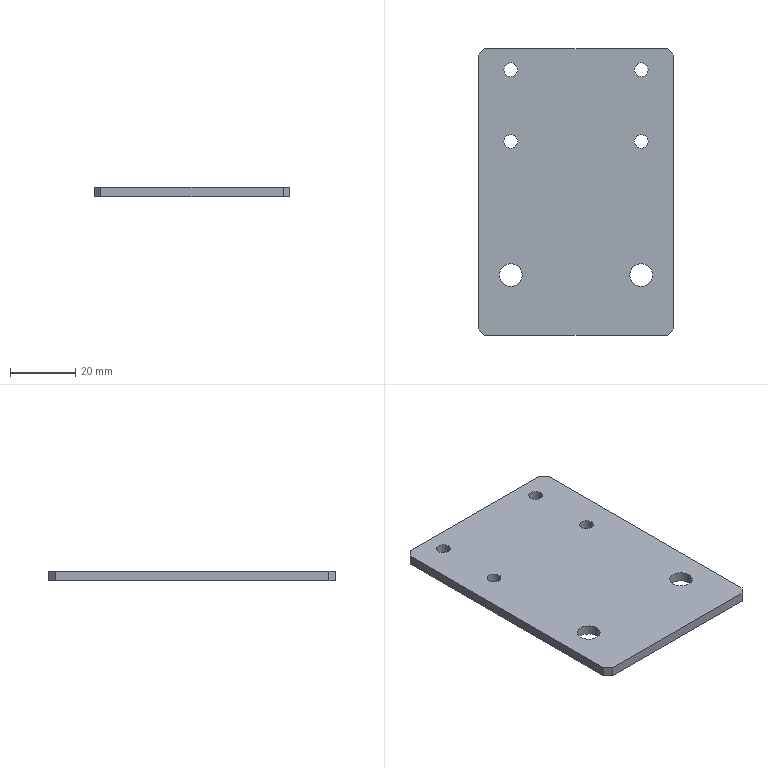Part | NX | features BREP 1 | 1 solid | 22 faces | box 60 x 88 x 3 mm | volume 15419 mm3 | cylinder 12 | plane 10 | commonest cylinder face diameters 4.2 x8 7 x4
STEP:
#1=CARTESIAN_POINT('',(30.,-42.,-3.));
#2=VERTEX_POINT('',#1);
#3=CARTESIAN_POINT('',(28.,-44.,-3.));
#4=VERTEX_POINT('',#3);
#5=CARTESIAN_POINT('',(28.,-44.,-3.));
#6=DIRECTION('',(-0.7071,-0.7071,0.));
#7=VECTOR('',#6,1000.);
#8=LINE('',#5,#7);
#9=EDGE_CURVE('',#2,#4,#8,.T.);
#10=ORIENTED_EDGE('',*,*,#9,.F.);
#11=CARTESIAN_POINT('',(30.,-42.,0.));
#12=VERTEX_POINT('',#11);
#13=CARTESIAN_POINT('',(30.,-42.,-3.));
#14=DIRECTION('',(0.,0.,-1.));
#15=VECTOR('',#14,1000.);
#16=LINE('',#13,#15);
#17=EDGE_CURVE('',#12,#2,#16,.T.);
#18=ORIENTED_EDGE('',*,*,#17,.F.);
#19=CARTESIAN_POINT('',(28.,-44.,0.));
#20=VERTEX_POINT('',#19);
#21=CARTESIAN_POINT('',(36.,-36.,0.));
#22=DIRECTION('',(0.7071,0.7071,0.));
#23=VECTOR('',#22,1000.);
#24=LINE('',#21,#23);
#25=EDGE_CURVE('',#20,#12,#24,.T.);
#26=ORIENTED_EDGE('',*,*,#25,.F.);
#27=CARTESIAN_POINT('',(28.,-44.,-3.));
#28=DIRECTION('',(0.,0.,1.));
#29=VECTOR('',#28,1000.);
#30=LINE('',#27,#29);
#31=EDGE_CURVE('',#4,#20,#30,.T.);
#32=ORIENTED_EDGE('',*,*,#31,.F.);
#33=EDGE_LOOP('',(#10,#18,#26,#32));
#34=FACE_BOUND('',#33,.T.);
#35=CARTESIAN_POINT('',(28.,-44.,-3.));
#36=DIRECTION('',(-0.7071,0.7071,0.));
#37=DIRECTION('',(0.,0.,1.));
#38=AXIS2_PLACEMENT_3D('',#35,#36,#37);
#39=PLANE('',#38);
#40=ADVANCED_FACE('',(#34),#39,.F.);
#41=CARTESIAN_POINT('',(-28.,-44.,-3.));
#42=VERTEX_POINT('',#41);
#43=CARTESIAN_POINT('',(-30.,-42.,-3.));
#44=VERTEX_POINT('',#43);
#45=CARTESIAN_POINT('',(-30.,-42.,-3.));
#46=DIRECTION('',(-0.7071,0.7071,0.));
#47=VECTOR('',#46,1000.);
#48=LINE('',#45,#47);
#49=EDGE_CURVE('',#42,#44,#48,.T.);
#50=ORIENTED_EDGE('',*,*,#49,.F.);
#51=CARTESIAN_POINT('',(-28.,-44.,0.));
#52=VERTEX_POINT('',#51);
#53=CARTESIAN_POINT('',(-28.,-44.,-3.));
#54=DIRECTION('',(0.,0.,-1.));
#55=VECTOR('',#54,1000.);
#56=LINE('',#53,#55);
#57=EDGE_CURVE('',#52,#42,#56,.T.);
#58=ORIENTED_EDGE('',*,*,#57,.F.);
#59=CARTESIAN_POINT('',(-30.,-42.,0.));
#60=VERTEX_POINT('',#59);
#61=CARTESIAN_POINT('',(-36.,-36.,0.));
#62=DIRECTION('',(0.7071,-0.7071,0.));
#63=VECTOR('',#62,1000.);
#64=LINE('',#61,#63);
#65=EDGE_CURVE('',#60,#52,#64,.T.);
#66=ORIENTED_EDGE('',*,*,#65,.F.);
#67=CARTESIAN_POINT('',(-30.,-42.,-3.));
#68=DIRECTION('',(0.,0.,1.));
#69=VECTOR('',#68,1000.);
#70=LINE('',#67,#69);
#71=EDGE_CURVE('',#44,#60,#70,.T.);
#72=ORIENTED_EDGE('',*,*,#71,.F.);
#73=EDGE_LOOP('',(#50,#58,#66,#72));
#74=FACE_BOUND('',#73,.T.);
#75=CARTESIAN_POINT('',(-30.,-42.,-3.));
#76=DIRECTION('',(0.7071,0.7071,0.));
#77=DIRECTION('',(0.,0.,1.));
#78=AXIS2_PLACEMENT_3D('',#75,#76,#77);
#79=PLANE('',#78);
#80=ADVANCED_FACE('',(#74),#79,.F.);
#81=CARTESIAN_POINT('',(28.,44.,-3.));
#82=VERTEX_POINT('',#81);
#83=CARTESIAN_POINT('',(30.,42.,-3.));
#84=VERTEX_POINT('',#83);
#85=CARTESIAN_POINT('',(30.,42.,-3.));
#86=DIRECTION('',(0.7071,-0.7071,0.));
#87=VECTOR('',#86,1000.);
#88=LINE('',#85,#87);
#89=EDGE_CURVE('',#82,#84,#88,.T.);
#90=ORIENTED_EDGE('',*,*,#89,.F.);
#91=CARTESIAN_POINT('',(28.,44.,0.));
#92=VERTEX_POINT('',#91);
#93=CARTESIAN_POINT('',(28.,44.,-3.));
#94=DIRECTION('',(0.,0.,-1.));
#95=VECTOR('',#94,1000.);
#96=LINE('',#93,#95);
#97=EDGE_CURVE('',#92,#82,#96,.T.);
#98=ORIENTED_EDGE('',*,*,#97,.F.);
#99=CARTESIAN_POINT('',(30.,42.,0.));
#100=VERTEX_POINT('',#99);
#101=CARTESIAN_POINT('',(36.,36.,0.));
#102=DIRECTION('',(-0.7071,0.7071,0.));
#103=VECTOR('',#102,1000.);
#104=LINE('',#101,#103);
#105=EDGE_CURVE('',#100,#92,#104,.T.);
#106=ORIENTED_EDGE('',*,*,#105,.F.);
#107=CARTESIAN_POINT('',(30.,42.,-3.));
#108=DIRECTION('',(0.,0.,1.));
#109=VECTOR('',#108,1000.);
#110=LINE('',#107,#109);
#111=EDGE_CURVE('',#84,#100,#110,.T.);
#112=ORIENTED_EDGE('',*,*,#111,.F.);
#113=EDGE_LOOP('',(#90,#98,#106,#112));
#114=FACE_BOUND('',#113,.T.);
#115=CARTESIAN_POINT('',(30.,42.,-3.));
#116=DIRECTION('',(-0.7071,-0.7071,0.));
#117=DIRECTION('',(0.,0.,1.));
#118=AXIS2_PLACEMENT_3D('',#115,#116,#117);
#119=PLANE('',#118);
#120=ADVANCED_FACE('',(#114),#119,.F.);
#121=CARTESIAN_POINT('',(-30.,42.,-3.));
#122=VERTEX_POINT('',#121);
#123=CARTESIAN_POINT('',(-28.,44.,-3.));
#124=VERTEX_POINT('',#123);
#125=CARTESIAN_POINT('',(-28.,44.,-3.));
#126=DIRECTION('',(0.7071,0.7071,0.));
#127=VECTOR('',#126,1000.);
#128=LINE('',#125,#127);
#129=EDGE_CURVE('',#122,#124,#128,.T.);
#130=ORIENTED_EDGE('',*,*,#129,.F.);
#131=CARTESIAN_POINT('',(-30.,42.,0.));
#132=VERTEX_POINT('',#131);
#133=CARTESIAN_POINT('',(-30.,42.,-3.));
#134=DIRECTION('',(0.,0.,-1.));
#135=VECTOR('',#134,1000.);
#136=LINE('',#133,#135);
#137=EDGE_CURVE('',#132,#122,#136,.T.);
#138=ORIENTED_EDGE('',*,*,#137,.F.);
#139=CARTESIAN_POINT('',(-28.,44.,0.));
#140=VERTEX_POINT('',#139);
#141=CARTESIAN_POINT('',(-36.,36.,0.));
#142=DIRECTION('',(-0.7071,-0.7071,0.));
#143=VECTOR('',#142,1000.);
#144=LINE('',#141,#143);
#145=EDGE_CURVE('',#140,#132,#144,.T.);
#146=ORIENTED_EDGE('',*,*,#145,.F.);
#147=CARTESIAN_POINT('',(-28.,44.,-3.));
#148=DIRECTION('',(0.,0.,1.));
#149=VECTOR('',#148,1000.);
#150=LINE('',#147,#149);
#151=EDGE_CURVE('',#124,#140,#150,.T.);
#152=ORIENTED_EDGE('',*,*,#151,.F.);
#153=EDGE_LOOP('',(#130,#138,#146,#152));
#154=FACE_BOUND('',#153,.T.);
#155=CARTESIAN_POINT('',(-28.,44.,-3.));
#156=DIRECTION('',(0.7071,-0.7071,0.));
#157=DIRECTION('',(0.,0.,1.));
#158=AXIS2_PLACEMENT_3D('',#155,#156,#157);
#159=PLANE('',#158);
#160=ADVANCED_FACE('',(#154),#159,.F.);
#161=CARTESIAN_POINT('',(23.5,-25.5,0.));
#162=VERTEX_POINT('',#161);
#163=CARTESIAN_POINT('',(23.5,-25.5,-3.));
#164=VERTEX_POINT('',#163);
#165=CARTESIAN_POINT('',(23.5,-25.5,-3.));
#166=DIRECTION('',(0.,0.,-1.));
#167=VECTOR('',#166,1000.);
#168=LINE('',#165,#167);
#169=EDGE_CURVE('',#162,#164,#168,.T.);
#170=ORIENTED_EDGE('',*,*,#169,.F.);
#171=CARTESIAN_POINT('',(16.5,-25.5,0.));
#172=VERTEX_POINT('',#171);
#173=CARTESIAN_POINT('',(20.,-25.5,0.));
#174=DIRECTION('',(0.,0.,-1.));
#175=DIRECTION('',(-1.,0.,0.));
#176=AXIS2_PLACEMENT_3D('',#173,#174,#175);
#177=CIRCLE('',#176,3.5);
#178=EDGE_CURVE('',#172,#162,#177,.T.);
#179=ORIENTED_EDGE('',*,*,#178,.F.);
#180=CARTESIAN_POINT('',(16.5,-25.5,-3.));
#181=VERTEX_POINT('',#180);
#182=CARTESIAN_POINT('',(16.5,-25.5,-3.));
#183=DIRECTION('',(0.,0.,-1.));
#184=VECTOR('',#183,1000.);
#185=LINE('',#182,#184);
#186=EDGE_CURVE('',#172,#181,#185,.T.);
#187=ORIENTED_EDGE('',*,*,#186,.T.);
#188=CARTESIAN_POINT('',(20.,-25.5,-3.));
#189=DIRECTION('',(0.,0.,-1.));
#190=DIRECTION('',(-1.,0.,0.));
#191=AXIS2_PLACEMENT_3D('',#188,#189,#190);
#192=CIRCLE('',#191,3.5);
#193=EDGE_CURVE('',#181,#164,#192,.T.);
#194=ORIENTED_EDGE('',*,*,#193,.T.);
#195=EDGE_LOOP('',(#170,#179,#187,#194));
#196=FACE_BOUND('',#195,.T.);
#197=CARTESIAN_POINT('',(20.,-25.5,-3.));
#198=DIRECTION('',(0.,0.,-1.));
#199=DIRECTION('',(-1.,0.,0.));
#200=AXIS2_PLACEMENT_3D('',#197,#198,#199);
#201=CYLINDRICAL_SURFACE('',#200,3.5);
#202=ADVANCED_FACE('',(#196),#201,.F.);
#203=CARTESIAN_POINT('',(-16.5,-25.5,0.));
#204=VERTEX_POINT('',#203);
#205=CARTESIAN_POINT('',(-16.5,-25.5,-3.));
#206=VERTEX_POINT('',#205);
#207=CARTESIAN_POINT('',(-16.5,-25.5,-3.));
#208=DIRECTION('',(0.,0.,-1.));
#209=VECTOR('',#208,1000.);
#210=LINE('',#207,#209);
#211=EDGE_CURVE('',#204,#206,#210,.T.);
#212=ORIENTED_EDGE('',*,*,#211,.F.);
#213=CARTESIAN_POINT('',(-23.5,-25.5,0.));
#214=VERTEX_POINT('',#213);
#215=CARTESIAN_POINT('',(-20.,-25.5,0.));
#216=DIRECTION('',(0.,0.,-1.));
#217=DIRECTION('',(-1.,0.,0.));
#218=AXIS2_PLACEMENT_3D('',#215,#216,#217);
#219=CIRCLE('',#218,3.5);
#220=EDGE_CURVE('',#214,#204,#219,.T.);
#221=ORIENTED_EDGE('',*,*,#220,.F.);
#222=CARTESIAN_POINT('',(-23.5,-25.5,-3.));
#223=VERTEX_POINT('',#222);
#224=CARTESIAN_POINT('',(-23.5,-25.5,-3.));
#225=DIRECTION('',(0.,0.,-1.));
#226=VECTOR('',#225,1000.);
#227=LINE('',#224,#226);
#228=EDGE_CURVE('',#214,#223,#227,.T.);
#229=ORIENTED_EDGE('',*,*,#228,.T.);
#230=CARTESIAN_POINT('',(-20.,-25.5,-3.));
#231=DIRECTION('',(0.,0.,-1.));
#232=DIRECTION('',(-1.,0.,0.));
#233=AXIS2_PLACEMENT_3D('',#230,#231,#232);
#234=CIRCLE('',#233,3.5);
#235=EDGE_CURVE('',#223,#206,#234,.T.);
#236=ORIENTED_EDGE('',*,*,#235,.T.);
#237=EDGE_LOOP('',(#212,#221,#229,#236));
#238=FACE_BOUND('',#237,.T.);
#239=CARTESIAN_POINT('',(-20.,-25.5,-3.));
#240=DIRECTION('',(0.,0.,-1.));
#241=DIRECTION('',(-1.,0.,0.));
#242=AXIS2_PLACEMENT_3D('',#239,#240,#241);
#243=CYLINDRICAL_SURFACE('',#242,3.5);
#244=ADVANCED_FACE('',(#238),#243,.F.);
#245=CARTESIAN_POINT('',(-17.9,15.5,0.));
#246=VERTEX_POINT('',#245);
#247=CARTESIAN_POINT('',(-17.9,15.5,-3.));
#248=VERTEX_POINT('',#247);
#249=CARTESIAN_POINT('',(-17.9,15.5,-3.));
#250=DIRECTION('',(0.,0.,-1.));
#251=VECTOR('',#250,1000.);
#252=LINE('',#249,#251);
#253=EDGE_CURVE('',#246,#248,#252,.T.);
#254=ORIENTED_EDGE('',*,*,#253,.F.);
#255=CARTESIAN_POINT('',(-22.1,15.5,0.));
#256=VERTEX_POINT('',#255);
#257=CARTESIAN_POINT('',(-20.,15.5,0.));
#258=DIRECTION('',(0.,0.,1.));
#259=DIRECTION('',(1.,0.,0.));
#260=AXIS2_PLACEMENT_3D('',#257,#258,#259);
#261=CIRCLE('',#260,2.1);
#262=EDGE_CURVE('',#246,#256,#261,.T.);
#263=ORIENTED_EDGE('',*,*,#262,.T.);
#264=CARTESIAN_POINT('',(-22.1,15.5,-3.));
#265=VERTEX_POINT('',#264);
#266=CARTESIAN_POINT('',(-22.1,15.5,-3.));
#267=DIRECTION('',(0.,0.,-1.));
#268=VECTOR('',#267,1000.);
#269=LINE('',#266,#268);
#270=EDGE_CURVE('',#256,#265,#269,.T.);
#271=ORIENTED_EDGE('',*,*,#270,.T.);
#272=CARTESIAN_POINT('',(-20.,15.5,-3.));
#273=DIRECTION('',(0.,0.,-1.));
#274=DIRECTION('',(-1.,0.,0.));
#275=AXIS2_PLACEMENT_3D('',#272,#273,#274);
#276=CIRCLE('',#275,2.1);
#277=EDGE_CURVE('',#265,#248,#276,.T.);
#278=ORIENTED_EDGE('',*,*,#277,.T.);
#279=EDGE_LOOP('',(#254,#263,#271,#278));
#280=FACE_BOUND('',#279,.T.);
#281=CARTESIAN_POINT('',(-20.,15.5,-3.));
#282=DIRECTION('',(0.,0.,-1.));
#283=DIRECTION('',(-1.,0.,0.));
#284=AXIS2_PLACEMENT_3D('',#281,#282,#283);
#285=CYLINDRICAL_SURFACE('',#284,2.1);
#286=ADVANCED_FACE('',(#280),#285,.F.);
#287=CARTESIAN_POINT('',(-17.9,37.5,0.));
#288=VERTEX_POINT('',#287);
#289=CARTESIAN_POINT('',(-17.9,37.5,-3.));
#290=VERTEX_POINT('',#289);
#291=CARTESIAN_POINT('',(-17.9,37.5,-3.));
#292=DIRECTION('',(0.,0.,-1.));
#293=VECTOR('',#292,1000.);
#294=LINE('',#291,#293);
#295=EDGE_CURVE('',#288,#290,#294,.T.);
#296=ORIENTED_EDGE('',*,*,#295,.F.);
#297=CARTESIAN_POINT('',(-22.1,37.5,0.));
#298=VERTEX_POINT('',#297);
#299=CARTESIAN_POINT('',(-20.,37.5,0.));
#300=DIRECTION('',(0.,0.,1.));
#301=DIRECTION('',(1.,0.,0.));
#302=AXIS2_PLACEMENT_3D('',#299,#300,#301);
#303=CIRCLE('',#302,2.1);
#304=EDGE_CURVE('',#288,#298,#303,.T.);
#305=ORIENTED_EDGE('',*,*,#304,.T.);
#306=CARTESIAN_POINT('',(-22.1,37.5,-3.));
#307=VERTEX_POINT('',#306);
#308=CARTESIAN_POINT('',(-22.1,37.5,-3.));
#309=DIRECTION('',(0.,0.,-1.));
#310=VECTOR('',#309,1000.);
#311=LINE('',#308,#310);
#312=EDGE_CURVE('',#298,#307,#311,.T.);
#313=ORIENTED_EDGE('',*,*,#312,.T.);
#314=CARTESIAN_POINT('',(-20.,37.5,-3.));
#315=DIRECTION('',(0.,0.,-1.));
#316=DIRECTION('',(-1.,0.,0.));
#317=AXIS2_PLACEMENT_3D('',#314,#315,#316);
#318=CIRCLE('',#317,2.1);
#319=EDGE_CURVE('',#307,#290,#318,.T.);
#320=ORIENTED_EDGE('',*,*,#319,.T.);
#321=EDGE_LOOP('',(#296,#305,#313,#320));
#322=FACE_BOUND('',#321,.T.);
#323=CARTESIAN_POINT('',(-20.,37.5,-3.));
#324=DIRECTION('',(0.,0.,-1.));
#325=DIRECTION('',(-1.,0.,0.));
#326=AXIS2_PLACEMENT_3D('',#323,#324,#325);
#327=CYLINDRICAL_SURFACE('',#326,2.1);
#328=ADVANCED_FACE('',(#322),#327,.F.);
#329=CARTESIAN_POINT('',(22.1,37.5,0.));
#330=VERTEX_POINT('',#329);
#331=CARTESIAN_POINT('',(22.1,37.5,-3.));
#332=VERTEX_POINT('',#331);
#333=CARTESIAN_POINT('',(22.1,37.5,-3.));
#334=DIRECTION('',(0.,0.,-1.));
#335=VECTOR('',#334,1000.);
#336=LINE('',#333,#335);
#337=EDGE_CURVE('',#330,#332,#336,.T.);
#338=ORIENTED_EDGE('',*,*,#337,.F.);
#339=CARTESIAN_POINT('',(17.9,37.5,0.));
#340=VERTEX_POINT('',#339);
#341=CARTESIAN_POINT('',(20.,37.5,0.));
#342=DIRECTION('',(0.,0.,1.));
#343=DIRECTION('',(1.,0.,0.));
#344=AXIS2_PLACEMENT_3D('',#341,#342,#343);
#345=CIRCLE('',#344,2.1);
#346=EDGE_CURVE('',#330,#340,#345,.T.);
#347=ORIENTED_EDGE('',*,*,#346,.T.);
#348=CARTESIAN_POINT('',(17.9,37.5,-3.));
#349=VERTEX_POINT('',#348);
#350=CARTESIAN_POINT('',(17.9,37.5,-3.));
#351=DIRECTION('',(0.,0.,-1.));
#352=VECTOR('',#351,1000.);
#353=LINE('',#350,#352);
#354=EDGE_CURVE('',#340,#349,#353,.T.);
#355=ORIENTED_EDGE('',*,*,#354,.T.);
#356=CARTESIAN_POINT('',(20.,37.5,-3.));
#357=DIRECTION('',(0.,0.,-1.));
#358=DIRECTION('',(-1.,0.,0.));
#359=AXIS2_PLACEMENT_3D('',#356,#357,#358);
#360=CIRCLE('',#359,2.1);
#361=EDGE_CURVE('',#349,#332,#360,.T.);
#362=ORIENTED_EDGE('',*,*,#361,.T.);
#363=EDGE_LOOP('',(#338,#347,#355,#362));
#364=FACE_BOUND('',#363,.T.);
#365=CARTESIAN_POINT('',(20.,37.5,-3.));
#366=DIRECTION('',(0.,0.,-1.));
#367=DIRECTION('',(-1.,0.,0.));
#368=AXIS2_PLACEMENT_3D('',#365,#366,#367);
#369=CYLINDRICAL_SURFACE('',#368,2.1);
#370=ADVANCED_FACE('',(#364),#369,.F.);
#371=CARTESIAN_POINT('',(22.1,15.5,0.));
#372=VERTEX_POINT('',#371);
#373=CARTESIAN_POINT('',(22.1,15.5,-3.));
#374=VERTEX_POINT('',#373);
#375=CARTESIAN_POINT('',(22.1,15.5,-3.));
#376=DIRECTION('',(0.,0.,-1.));
#377=VECTOR('',#376,1000.);
#378=LINE('',#375,#377);
#379=EDGE_CURVE('',#372,#374,#378,.T.);
#380=ORIENTED_EDGE('',*,*,#379,.F.);
#381=CARTESIAN_POINT('',(17.9,15.5,0.));
#382=VERTEX_POINT('',#381);
#383=CARTESIAN_POINT('',(20.,15.5,0.));
#384=DIRECTION('',(0.,0.,1.));
#385=DIRECTION('',(1.,0.,0.));
#386=AXIS2_PLACEMENT_3D('',#383,#384,#385);
#387=CIRCLE('',#386,2.1);
#388=EDGE_CURVE('',#372,#382,#387,.T.);
#389=ORIENTED_EDGE('',*,*,#388,.T.);
#390=CARTESIAN_POINT('',(17.9,15.5,-3.));
#391=VERTEX_POINT('',#390);
#392=CARTESIAN_POINT('',(17.9,15.5,-3.));
#393=DIRECTION('',(0.,0.,-1.));
#394=VECTOR('',#393,1000.);
#395=LINE('',#392,#394);
#396=EDGE_CURVE('',#382,#391,#395,.T.);
#397=ORIENTED_EDGE('',*,*,#396,.T.);
#398=CARTESIAN_POINT('',(20.,15.5,-3.));
#399=DIRECTION('',(0.,0.,-1.));
#400=DIRECTION('',(-1.,0.,0.));
#401=AXIS2_PLACEMENT_3D('',#398,#399,#400);
#402=CIRCLE('',#401,2.1);
#403=EDGE_CURVE('',#391,#374,#402,.T.);
#404=ORIENTED_EDGE('',*,*,#403,.T.);
#405=EDGE_LOOP('',(#380,#389,#397,#404));
#406=FACE_BOUND('',#405,.T.);
#407=CARTESIAN_POINT('',(20.,15.5,-3.));
#408=DIRECTION('',(0.,0.,-1.));
#409=DIRECTION('',(-1.,0.,0.));
#410=AXIS2_PLACEMENT_3D('',#407,#408,#409);
#411=CYLINDRICAL_SURFACE('',#410,2.1);
#412=ADVANCED_FACE('',(#406),#411,.F.);
#413=CARTESIAN_POINT('',(-30.,44.,0.));
#414=DIRECTION('',(-1.,0.,0.));
#415=VECTOR('',#414,1000.);
#416=LINE('',#413,#415);
#417=EDGE_CURVE('',#92,#140,#416,.T.);
#418=ORIENTED_EDGE('',*,*,#417,.T.);
#419=ORIENTED_EDGE('',*,*,#145,.T.);
#420=CARTESIAN_POINT('',(-30.,44.,0.));
#421=DIRECTION('',(0.,-1.,0.));
#422=VECTOR('',#421,1000.);
#423=LINE('',#420,#422);
#424=EDGE_CURVE('',#132,#60,#423,.T.);
#425=ORIENTED_EDGE('',*,*,#424,.T.);
#426=ORIENTED_EDGE('',*,*,#65,.T.);
#427=CARTESIAN_POINT('',(-30.,-44.,0.));
#428=DIRECTION('',(1.,0.,0.));
#429=VECTOR('',#428,1000.);
#430=LINE('',#427,#429);
#431=EDGE_CURVE('',#52,#20,#430,.T.);
#432=ORIENTED_EDGE('',*,*,#431,.T.);
#433=ORIENTED_EDGE('',*,*,#25,.T.);
#434=CARTESIAN_POINT('',(30.,44.,0.));
#435=DIRECTION('',(0.,1.,0.));
#436=VECTOR('',#435,1000.);
#437=LINE('',#434,#436);
#438=EDGE_CURVE('',#12,#100,#437,.T.);
#439=ORIENTED_EDGE('',*,*,#438,.T.);
#440=ORIENTED_EDGE('',*,*,#105,.T.);
#441=EDGE_LOOP('',(#418,#419,#425,#426,#432,#433,#439,#440));
#442=FACE_BOUND('',#441,.T.);
#443=CARTESIAN_POINT('',(20.,15.5,0.));
#444=DIRECTION('',(0.,0.,1.));
#445=DIRECTION('',(1.,0.,0.));
#446=AXIS2_PLACEMENT_3D('',#443,#444,#445);
#447=CIRCLE('',#446,2.1);
#448=EDGE_CURVE('',#382,#372,#447,.T.);
#449=ORIENTED_EDGE('',*,*,#448,.F.);
#450=ORIENTED_EDGE('',*,*,#388,.F.);
#451=EDGE_LOOP('',(#449,#450));
#452=FACE_BOUND('',#451,.T.);
#453=CARTESIAN_POINT('',(20.,37.5,0.));
#454=DIRECTION('',(0.,0.,1.));
#455=DIRECTION('',(1.,0.,0.));
#456=AXIS2_PLACEMENT_3D('',#453,#454,#455);
#457=CIRCLE('',#456,2.1);
#458=EDGE_CURVE('',#340,#330,#457,.T.);
#459=ORIENTED_EDGE('',*,*,#458,.F.);
#460=ORIENTED_EDGE('',*,*,#346,.F.);
#461=EDGE_LOOP('',(#459,#460));
#462=FACE_BOUND('',#461,.T.);
#463=CARTESIAN_POINT('',(-20.,37.5,0.));
#464=DIRECTION('',(0.,0.,1.));
#465=DIRECTION('',(1.,0.,0.));
#466=AXIS2_PLACEMENT_3D('',#463,#464,#465);
#467=CIRCLE('',#466,2.1);
#468=EDGE_CURVE('',#298,#288,#467,.T.);
#469=ORIENTED_EDGE('',*,*,#468,.F.);
#470=ORIENTED_EDGE('',*,*,#304,.F.);
#471=EDGE_LOOP('',(#469,#470));
#472=FACE_BOUND('',#471,.T.);
#473=CARTESIAN_POINT('',(-20.,15.5,0.));
#474=DIRECTION('',(0.,0.,1.));
#475=DIRECTION('',(1.,0.,0.));
#476=AXIS2_PLACEMENT_3D('',#473,#474,#475);
#477=CIRCLE('',#476,2.1);
#478=EDGE_CURVE('',#256,#246,#477,.T.);
#479=ORIENTED_EDGE('',*,*,#478,.F.);
#480=ORIENTED_EDGE('',*,*,#262,.F.);
#481=EDGE_LOOP('',(#479,#480));
#482=FACE_BOUND('',#481,.T.);
#483=ORIENTED_EDGE('',*,*,#220,.T.);
#484=CARTESIAN_POINT('',(-20.,-25.5,0.));
#485=DIRECTION('',(0.,0.,-1.));
#486=DIRECTION('',(-1.,0.,0.));
#487=AXIS2_PLACEMENT_3D('',#484,#485,#486);
#488=CIRCLE('',#487,3.5);
#489=EDGE_CURVE('',#204,#214,#488,.T.);
#490=ORIENTED_EDGE('',*,*,#489,.T.);
#491=EDGE_LOOP('',(#483,#490));
#492=FACE_BOUND('',#491,.T.);
#493=ORIENTED_EDGE('',*,*,#178,.T.);
#494=CARTESIAN_POINT('',(20.,-25.5,0.));
#495=DIRECTION('',(0.,0.,-1.));
#496=DIRECTION('',(-1.,0.,0.));
#497=AXIS2_PLACEMENT_3D('',#494,#495,#496);
#498=CIRCLE('',#497,3.5);
#499=EDGE_CURVE('',#162,#172,#498,.T.);
#500=ORIENTED_EDGE('',*,*,#499,.T.);
#501=EDGE_LOOP('',(#493,#500));
#502=FACE_BOUND('',#501,.T.);
#503=CARTESIAN_POINT('',(0.,0.,0.));
#504=DIRECTION('',(0.,0.,1.));
#505=DIRECTION('',(1.,0.,0.));
#506=AXIS2_PLACEMENT_3D('',#503,#504,#505);
#507=PLANE('',#506);
#508=ADVANCED_FACE('',(#442,#452,#462,#472,#482,#492,#502),#507,.T.);
#509=CARTESIAN_POINT('',(-30.,44.,-3.));
#510=DIRECTION('',(0.,-1.,0.));
#511=VECTOR('',#510,1000.);
#512=LINE('',#509,#511);
#513=EDGE_CURVE('',#122,#44,#512,.T.);
#514=ORIENTED_EDGE('',*,*,#513,.F.);
#515=ORIENTED_EDGE('',*,*,#129,.T.);
#516=CARTESIAN_POINT('',(-30.,44.,-3.));
#517=DIRECTION('',(-1.,0.,0.));
#518=VECTOR('',#517,1000.);
#519=LINE('',#516,#518);
#520=EDGE_CURVE('',#82,#124,#519,.T.);
#521=ORIENTED_EDGE('',*,*,#520,.F.);
#522=ORIENTED_EDGE('',*,*,#89,.T.);
#523=CARTESIAN_POINT('',(30.,44.,-3.));
#524=DIRECTION('',(0.,1.,0.));
#525=VECTOR('',#524,1000.);
#526=LINE('',#523,#525);
#527=EDGE_CURVE('',#2,#84,#526,.T.);
#528=ORIENTED_EDGE('',*,*,#527,.F.);
#529=ORIENTED_EDGE('',*,*,#9,.T.);
#530=CARTESIAN_POINT('',(-30.,-44.,-3.));
#531=DIRECTION('',(1.,0.,0.));
#532=VECTOR('',#531,1000.);
#533=LINE('',#530,#532);
#534=EDGE_CURVE('',#42,#4,#533,.T.);
#535=ORIENTED_EDGE('',*,*,#534,.F.);
#536=ORIENTED_EDGE('',*,*,#49,.T.);
#537=EDGE_LOOP('',(#514,#515,#521,#522,#528,#529,#535,#536));
#538=FACE_BOUND('',#537,.T.);
#539=ORIENTED_EDGE('',*,*,#403,.F.);
#540=CARTESIAN_POINT('',(20.,15.5,-3.));
#541=DIRECTION('',(0.,0.,-1.));
#542=DIRECTION('',(-1.,0.,0.));
#543=AXIS2_PLACEMENT_3D('',#540,#541,#542);
#544=CIRCLE('',#543,2.1);
#545=EDGE_CURVE('',#374,#391,#544,.T.);
#546=ORIENTED_EDGE('',*,*,#545,.F.);
#547=EDGE_LOOP('',(#539,#546));
#548=FACE_BOUND('',#547,.T.);
#549=ORIENTED_EDGE('',*,*,#361,.F.);
#550=CARTESIAN_POINT('',(20.,37.5,-3.));
#551=DIRECTION('',(0.,0.,-1.));
#552=DIRECTION('',(-1.,0.,0.));
#553=AXIS2_PLACEMENT_3D('',#550,#551,#552);
#554=CIRCLE('',#553,2.1);
#555=EDGE_CURVE('',#332,#349,#554,.T.);
#556=ORIENTED_EDGE('',*,*,#555,.F.);
#557=EDGE_LOOP('',(#549,#556));
#558=FACE_BOUND('',#557,.T.);
#559=ORIENTED_EDGE('',*,*,#319,.F.);
#560=CARTESIAN_POINT('',(-20.,37.5,-3.));
#561=DIRECTION('',(0.,0.,-1.));
#562=DIRECTION('',(-1.,0.,0.));
#563=AXIS2_PLACEMENT_3D('',#560,#561,#562);
#564=CIRCLE('',#563,2.1);
#565=EDGE_CURVE('',#290,#307,#564,.T.);
#566=ORIENTED_EDGE('',*,*,#565,.F.);
#567=EDGE_LOOP('',(#559,#566));
#568=FACE_BOUND('',#567,.T.);
#569=ORIENTED_EDGE('',*,*,#277,.F.);
#570=CARTESIAN_POINT('',(-20.,15.5,-3.));
#571=DIRECTION('',(0.,0.,-1.));
#572=DIRECTION('',(-1.,0.,0.));
#573=AXIS2_PLACEMENT_3D('',#570,#571,#572);
#574=CIRCLE('',#573,2.1);
#575=EDGE_CURVE('',#248,#265,#574,.T.);
#576=ORIENTED_EDGE('',*,*,#575,.F.);
#577=EDGE_LOOP('',(#569,#576));
#578=FACE_BOUND('',#577,.T.);
#579=ORIENTED_EDGE('',*,*,#235,.F.);
#580=CARTESIAN_POINT('',(-20.,-25.5,-3.));
#581=DIRECTION('',(0.,0.,-1.));
#582=DIRECTION('',(-1.,0.,0.));
#583=AXIS2_PLACEMENT_3D('',#580,#581,#582);
#584=CIRCLE('',#583,3.5);
#585=EDGE_CURVE('',#206,#223,#584,.T.);
#586=ORIENTED_EDGE('',*,*,#585,.F.);
#587=EDGE_LOOP('',(#579,#586));
#588=FACE_BOUND('',#587,.T.);
#589=ORIENTED_EDGE('',*,*,#193,.F.);
#590=CARTESIAN_POINT('',(20.,-25.5,-3.));
#591=DIRECTION('',(0.,0.,-1.));
#592=DIRECTION('',(-1.,0.,0.));
#593=AXIS2_PLACEMENT_3D('',#590,#591,#592);
#594=CIRCLE('',#593,3.5);
#595=EDGE_CURVE('',#164,#181,#594,.T.);
#596=ORIENTED_EDGE('',*,*,#595,.F.);
#597=EDGE_LOOP('',(#589,#596));
#598=FACE_BOUND('',#597,.T.);
#599=CARTESIAN_POINT('',(0.,0.,-3.));
#600=DIRECTION('',(0.,0.,1.));
#601=DIRECTION('',(1.,0.,0.));
#602=AXIS2_PLACEMENT_3D('',#599,#600,#601);
#603=PLANE('',#602);
#604=ADVANCED_FACE('',(#538,#548,#558,#568,#578,#588,#598),#603,.F.);
#605=ORIENTED_EDGE('',*,*,#520,.T.);
#606=ORIENTED_EDGE('',*,*,#151,.T.);
#607=ORIENTED_EDGE('',*,*,#417,.F.);
#608=ORIENTED_EDGE('',*,*,#97,.T.);
#609=EDGE_LOOP('',(#605,#606,#607,#608));
#610=FACE_BOUND('',#609,.T.);
#611=CARTESIAN_POINT('',(-30.,44.,-3.));
#612=DIRECTION('',(0.,1.,0.));
#613=DIRECTION('',(0.,0.,1.));
#614=AXIS2_PLACEMENT_3D('',#611,#612,#613);
#615=PLANE('',#614);
#616=ADVANCED_FACE('',(#610),#615,.T.);
#617=ORIENTED_EDGE('',*,*,#424,.F.);
#618=ORIENTED_EDGE('',*,*,#137,.T.);
#619=ORIENTED_EDGE('',*,*,#513,.T.);
#620=ORIENTED_EDGE('',*,*,#71,.T.);
#621=EDGE_LOOP('',(#617,#618,#619,#620));
#622=FACE_BOUND('',#621,.T.);
#623=CARTESIAN_POINT('',(-30.,44.,-3.));
#624=DIRECTION('',(-1.,0.,0.));
#625=DIRECTION('',(0.,-1.,0.));
#626=AXIS2_PLACEMENT_3D('',#623,#624,#625);
#627=PLANE('',#626);
#628=ADVANCED_FACE('',(#622),#627,.T.);
#629=ORIENTED_EDGE('',*,*,#431,.F.);
#630=ORIENTED_EDGE('',*,*,#57,.T.);
#631=ORIENTED_EDGE('',*,*,#534,.T.);
#632=ORIENTED_EDGE('',*,*,#31,.T.);
#633=EDGE_LOOP('',(#629,#630,#631,#632));
#634=FACE_BOUND('',#633,.T.);
#635=CARTESIAN_POINT('',(-30.,-44.,-3.));
#636=DIRECTION('',(0.,-1.,0.));
#637=DIRECTION('',(0.,0.,-1.));
#638=AXIS2_PLACEMENT_3D('',#635,#636,#637);
#639=PLANE('',#638);
#640=ADVANCED_FACE('',(#634),#639,.T.);
#641=ORIENTED_EDGE('',*,*,#527,.T.);
#642=ORIENTED_EDGE('',*,*,#111,.T.);
#643=ORIENTED_EDGE('',*,*,#438,.F.);
#644=ORIENTED_EDGE('',*,*,#17,.T.);
#645=EDGE_LOOP('',(#641,#642,#643,#644));
#646=FACE_BOUND('',#645,.T.);
#647=CARTESIAN_POINT('',(30.,44.,-3.));
#648=DIRECTION('',(1.,0.,0.));
#649=DIRECTION('',(0.,1.,0.));
#650=AXIS2_PLACEMENT_3D('',#647,#648,#649);
#651=PLANE('',#650);
#652=ADVANCED_FACE('',(#646),#651,.T.);
#653=ORIENTED_EDGE('',*,*,#448,.T.);
#654=ORIENTED_EDGE('',*,*,#379,.T.);
#655=ORIENTED_EDGE('',*,*,#545,.T.);
#656=ORIENTED_EDGE('',*,*,#396,.F.);
#657=EDGE_LOOP('',(#653,#654,#655,#656));
#658=FACE_BOUND('',#657,.T.);
#659=CARTESIAN_POINT('',(20.,15.5,-3.));
#660=DIRECTION('',(0.,0.,-1.));
#661=DIRECTION('',(-1.,0.,0.));
#662=AXIS2_PLACEMENT_3D('',#659,#660,#661);
#663=CYLINDRICAL_SURFACE('',#662,2.1);
#664=ADVANCED_FACE('',(#658),#663,.F.);
#665=ORIENTED_EDGE('',*,*,#458,.T.);
#666=ORIENTED_EDGE('',*,*,#337,.T.);
#667=ORIENTED_EDGE('',*,*,#555,.T.);
#668=ORIENTED_EDGE('',*,*,#354,.F.);
#669=EDGE_LOOP('',(#665,#666,#667,#668));
#670=FACE_BOUND('',#669,.T.);
#671=CARTESIAN_POINT('',(20.,37.5,-3.));
#672=DIRECTION('',(0.,0.,-1.));
#673=DIRECTION('',(-1.,0.,0.));
#674=AXIS2_PLACEMENT_3D('',#671,#672,#673);
#675=CYLINDRICAL_SURFACE('',#674,2.1);
#676=ADVANCED_FACE('',(#670),#675,.F.);
#677=ORIENTED_EDGE('',*,*,#468,.T.);
#678=ORIENTED_EDGE('',*,*,#295,.T.);
#679=ORIENTED_EDGE('',*,*,#565,.T.);
#680=ORIENTED_EDGE('',*,*,#312,.F.);
#681=EDGE_LOOP('',(#677,#678,#679,#680));
#682=FACE_BOUND('',#681,.T.);
#683=CARTESIAN_POINT('',(-20.,37.5,-3.));
#684=DIRECTION('',(0.,0.,-1.));
#685=DIRECTION('',(-1.,0.,0.));
#686=AXIS2_PLACEMENT_3D('',#683,#684,#685);
#687=CYLINDRICAL_SURFACE('',#686,2.1);
#688=ADVANCED_FACE('',(#682),#687,.F.);
#689=ORIENTED_EDGE('',*,*,#478,.T.);
#690=ORIENTED_EDGE('',*,*,#253,.T.);
#691=ORIENTED_EDGE('',*,*,#575,.T.);
#692=ORIENTED_EDGE('',*,*,#270,.F.);
#693=EDGE_LOOP('',(#689,#690,#691,#692));
#694=FACE_BOUND('',#693,.T.);
#695=CARTESIAN_POINT('',(-20.,15.5,-3.));
#696=DIRECTION('',(0.,0.,-1.));
#697=DIRECTION('',(-1.,0.,0.));
#698=AXIS2_PLACEMENT_3D('',#695,#696,#697);
#699=CYLINDRICAL_SURFACE('',#698,2.1);
#700=ADVANCED_FACE('',(#694),#699,.F.);
#701=ORIENTED_EDGE('',*,*,#489,.F.);
#702=ORIENTED_EDGE('',*,*,#211,.T.);
#703=ORIENTED_EDGE('',*,*,#585,.T.);
#704=ORIENTED_EDGE('',*,*,#228,.F.);
#705=EDGE_LOOP('',(#701,#702,#703,#704));
#706=FACE_BOUND('',#705,.T.);
#707=CARTESIAN_POINT('',(-20.,-25.5,-3.));
#708=DIRECTION('',(0.,0.,-1.));
#709=DIRECTION('',(-1.,0.,0.));
#710=AXIS2_PLACEMENT_3D('',#707,#708,#709);
#711=CYLINDRICAL_SURFACE('',#710,3.5);
#712=ADVANCED_FACE('',(#706),#711,.F.);
#713=ORIENTED_EDGE('',*,*,#499,.F.);
#714=ORIENTED_EDGE('',*,*,#169,.T.);
#715=ORIENTED_EDGE('',*,*,#595,.T.);
#716=ORIENTED_EDGE('',*,*,#186,.F.);
#717=EDGE_LOOP('',(#713,#714,#715,#716));
#718=FACE_BOUND('',#717,.T.);
#719=CARTESIAN_POINT('',(20.,-25.5,-3.));
#720=DIRECTION('',(0.,0.,-1.));
#721=DIRECTION('',(-1.,0.,0.));
#722=AXIS2_PLACEMENT_3D('',#719,#720,#721);
#723=CYLINDRICAL_SURFACE('',#722,3.5);
#724=ADVANCED_FACE('',(#718),#723,.F.);
#725=CLOSED_SHELL('',(#40,#80,#120,#160,#202,#244,#286,#328,#370,#412,#508,#604,#616,#628,#640,#652,#664,#676,#688,#700,#712,#724));
#726=MANIFOLD_SOLID_BREP('',#725);
#727=(LENGTH_UNIT()NAMED_UNIT(*)SI_UNIT(.MILLI.,.METRE.));
#728=UNCERTAINTY_MEASURE_WITH_UNIT(LENGTH_MEASURE(0.00001),#727,'','');
#729=(NAMED_UNIT(*)PLANE_ANGLE_UNIT()SI_UNIT($,.RADIAN.));
#730=(NAMED_UNIT(*)SI_UNIT($,.STERADIAN.)SOLID_ANGLE_UNIT());
#731=(GEOMETRIC_REPRESENTATION_CONTEXT(3)GLOBAL_UNCERTAINTY_ASSIGNED_CONTEXT((#728))GLOBAL_UNIT_ASSIGNED_CONTEXT((#727,#729,#730))REPRESENTATION_CONTEXT('',''));
#732=ADVANCED_BREP_SHAPE_REPRESENTATION('',(#726),#731);